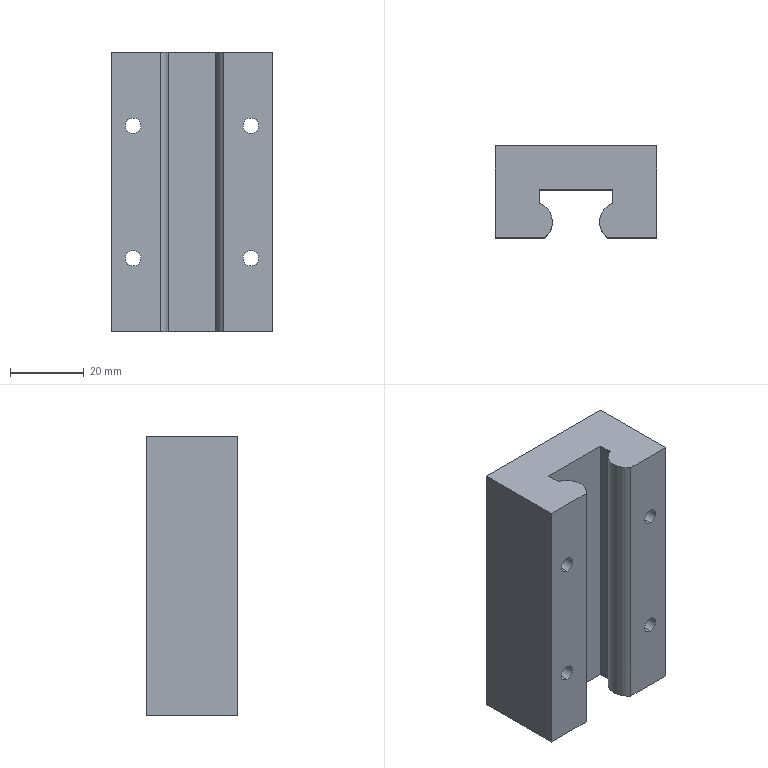Part | STEP file | Linear slider HGH20CA V1.201001 | 1 solid | 21 faces | box 44 x 25 x 76 mm | volume 66387 mm3 | cylinder 11 | plane 10 | commonest cylinder face diameters 4.2 x8 10.692 x3